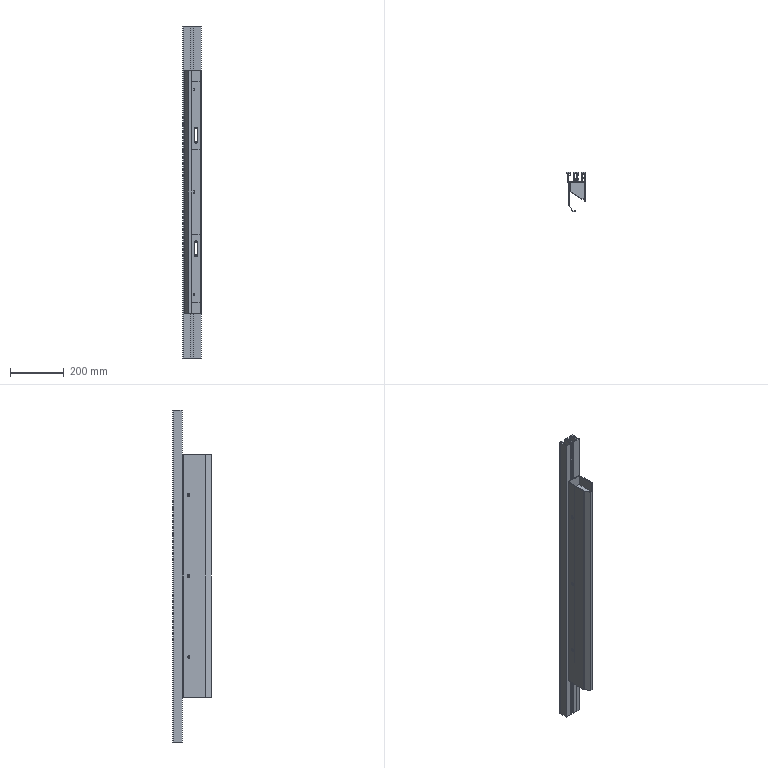Part | 7 solids | 239 faces | box 70 x 143.651 x 1230 mm | volume 1417083 mm3 | plane 164 | cylinder 75 | commonest cylinder face diameters 10 x19 7 x12 9 x12 2 x8 3 x5 5 x4